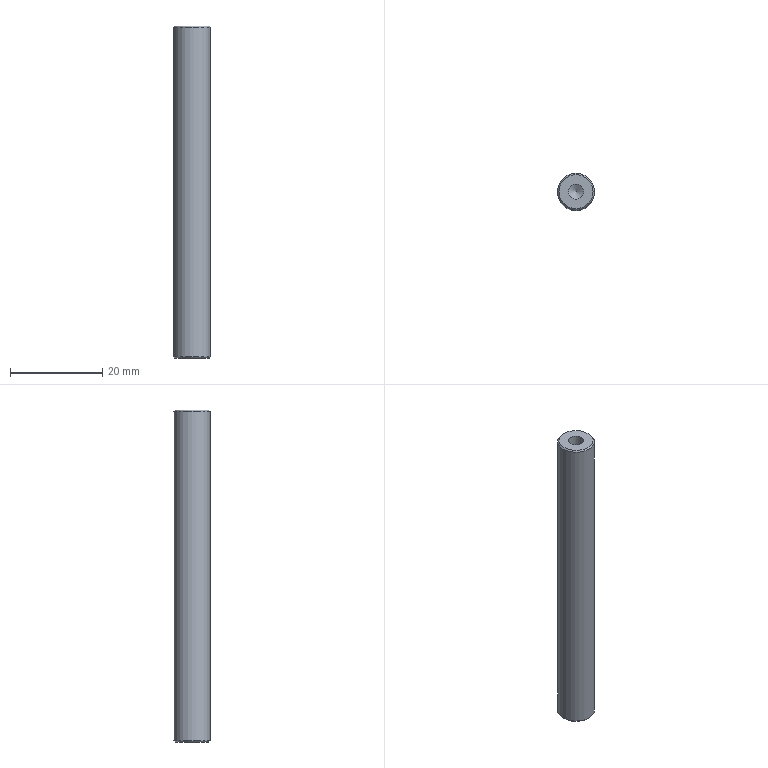Part | NX | 1 solid | 9 faces | box 8 x 8 x 72 mm | volume 3415 mm3 | cone 4 | cylinder 3 | plane 2 | commonest cylinder face diameters 3.3 x2 8 x1
STEP:
#1=CARTESIAN_POINT('',(4.,0.,35.7));
#2=VERTEX_POINT('',#1);
#3=CARTESIAN_POINT('',(0.,0.,35.7));
#4=DIRECTION('',(0.,0.,1.));
#5=DIRECTION('',(1.,0.,0.));
#6=AXIS2_PLACEMENT_3D('',#3,#4,#5);
#7=CIRCLE('',#6,4.);
#8=EDGE_CURVE('',#2,#2,#7,.F.);
#9=ORIENTED_EDGE('',*,*,#8,.T.);
#10=EDGE_LOOP('',(#9));
#11=FACE_BOUND('',#10,.T.);
#12=CARTESIAN_POINT('',(4.,0.,-35.7));
#13=VERTEX_POINT('',#12);
#14=CARTESIAN_POINT('',(0.,0.,-35.7));
#15=DIRECTION('',(0.,0.,1.));
#16=DIRECTION('',(1.,0.,0.));
#17=AXIS2_PLACEMENT_3D('',#14,#15,#16);
#18=CIRCLE('',#17,4.);
#19=EDGE_CURVE('',#13,#13,#18,.T.);
#20=ORIENTED_EDGE('',*,*,#19,.T.);
#21=EDGE_LOOP('',(#20));
#22=FACE_BOUND('',#21,.T.);
#23=CARTESIAN_POINT('',(0.,0.,36.));
#24=DIRECTION('',(0.,0.,-1.));
#25=DIRECTION('',(-1.,0.,0.));
#26=AXIS2_PLACEMENT_3D('',#23,#24,#25);
#27=CYLINDRICAL_SURFACE('',#26,4.);
#28=ADVANCED_FACE('',(#11,#22),#27,.T.);
#29=CARTESIAN_POINT('',(3.7,0.,36.));
#30=VERTEX_POINT('',#29);
#31=CARTESIAN_POINT('',(0.,0.,36.));
#32=DIRECTION('',(0.,0.,1.));
#33=DIRECTION('',(1.,0.,0.));
#34=AXIS2_PLACEMENT_3D('',#31,#32,#33);
#35=CIRCLE('',#34,3.7);
#36=EDGE_CURVE('',#30,#30,#35,.T.);
#37=ORIENTED_EDGE('',*,*,#36,.T.);
#38=EDGE_LOOP('',(#37));
#39=FACE_BOUND('',#38,.T.);
#40=CARTESIAN_POINT('',(1.65,0.,36.));
#41=VERTEX_POINT('',#40);
#42=CARTESIAN_POINT('',(0.,0.,36.));
#43=DIRECTION('',(0.,0.,1.));
#44=DIRECTION('',(1.,0.,0.));
#45=AXIS2_PLACEMENT_3D('',#42,#43,#44);
#46=CIRCLE('',#45,1.65);
#47=EDGE_CURVE('',#41,#41,#46,.T.);
#48=ORIENTED_EDGE('',*,*,#47,.F.);
#49=EDGE_LOOP('',(#48));
#50=FACE_BOUND('',#49,.T.);
#51=CARTESIAN_POINT('',(0.,0.,36.));
#52=DIRECTION('',(0.,0.,1.));
#53=DIRECTION('',(1.,0.,0.));
#54=AXIS2_PLACEMENT_3D('',#51,#52,#53);
#55=PLANE('',#54);
#56=ADVANCED_FACE('',(#39,#50),#55,.T.);
#57=CARTESIAN_POINT('',(3.7,0.,-36.));
#58=VERTEX_POINT('',#57);
#59=CARTESIAN_POINT('',(0.,0.,-36.));
#60=DIRECTION('',(0.,0.,1.));
#61=DIRECTION('',(1.,0.,0.));
#62=AXIS2_PLACEMENT_3D('',#59,#60,#61);
#63=CIRCLE('',#62,3.7);
#64=EDGE_CURVE('',#58,#58,#63,.F.);
#65=ORIENTED_EDGE('',*,*,#64,.T.);
#66=EDGE_LOOP('',(#65));
#67=FACE_BOUND('',#66,.T.);
#68=CARTESIAN_POINT('',(-1.65,0.,-36.));
#69=VERTEX_POINT('',#68);
#70=CARTESIAN_POINT('',(0.,0.,-36.));
#71=DIRECTION('',(0.,0.,-1.));
#72=DIRECTION('',(-1.,0.,0.));
#73=AXIS2_PLACEMENT_3D('',#70,#71,#72);
#74=CIRCLE('',#73,1.65);
#75=EDGE_CURVE('',#69,#69,#74,.T.);
#76=ORIENTED_EDGE('',*,*,#75,.F.);
#77=EDGE_LOOP('',(#76));
#78=FACE_BOUND('',#77,.T.);
#79=CARTESIAN_POINT('',(0.,0.,-36.));
#80=DIRECTION('',(0.,0.,1.));
#81=DIRECTION('',(1.,0.,0.));
#82=AXIS2_PLACEMENT_3D('',#79,#80,#81);
#83=PLANE('',#82);
#84=ADVANCED_FACE('',(#67,#78),#83,.F.);
#85=CARTESIAN_POINT('',(0.,0.,-23.509));
#86=VERTEX_POINT('',#85);
#87=VERTEX_LOOP('',#86);
#88=FACE_BOUND('',#87,.T.);
#89=CARTESIAN_POINT('',(-1.65,0.,-24.5));
#90=VERTEX_POINT('',#89);
#91=CARTESIAN_POINT('',(0.,0.,-24.5));
#92=DIRECTION('',(0.,0.,-1.));
#93=DIRECTION('',(-1.,0.,0.));
#94=AXIS2_PLACEMENT_3D('',#91,#92,#93);
#95=CIRCLE('',#94,1.65);
#96=EDGE_CURVE('',#90,#90,#95,.T.);
#97=ORIENTED_EDGE('',*,*,#96,.T.);
#98=EDGE_LOOP('',(#97));
#99=FACE_BOUND('',#98,.T.);
#100=CARTESIAN_POINT('',(0.,0.,-24.5));
#101=DIRECTION('',(0.,0.,-1.));
#102=DIRECTION('',(-1.,0.,0.));
#103=AXIS2_PLACEMENT_3D('',#100,#101,#102);
#104=CONICAL_SURFACE('',#103,1.65,1.03);
#105=ADVANCED_FACE('',(#88,#99),#104,.F.);
#106=ORIENTED_EDGE('',*,*,#96,.F.);
#107=EDGE_LOOP('',(#106));
#108=FACE_BOUND('',#107,.T.);
#109=ORIENTED_EDGE('',*,*,#75,.T.);
#110=EDGE_LOOP('',(#109));
#111=FACE_BOUND('',#110,.T.);
#112=CARTESIAN_POINT('',(0.,0.,-36.));
#113=DIRECTION('',(0.,0.,-1.));
#114=DIRECTION('',(-1.,0.,0.));
#115=AXIS2_PLACEMENT_3D('',#112,#113,#114);
#116=CYLINDRICAL_SURFACE('',#115,1.65);
#117=ADVANCED_FACE('',(#108,#111),#116,.F.);
#118=CARTESIAN_POINT('',(0.,0.,23.509));
#119=VERTEX_POINT('',#118);
#120=VERTEX_LOOP('',#119);
#121=FACE_BOUND('',#120,.T.);
#122=CARTESIAN_POINT('',(1.65,0.,24.5));
#123=VERTEX_POINT('',#122);
#124=CARTESIAN_POINT('',(0.,0.,24.5));
#125=DIRECTION('',(0.,0.,1.));
#126=DIRECTION('',(1.,0.,0.));
#127=AXIS2_PLACEMENT_3D('',#124,#125,#126);
#128=CIRCLE('',#127,1.65);
#129=EDGE_CURVE('',#123,#123,#128,.T.);
#130=ORIENTED_EDGE('',*,*,#129,.T.);
#131=EDGE_LOOP('',(#130));
#132=FACE_BOUND('',#131,.T.);
#133=CARTESIAN_POINT('',(0.,0.,24.5));
#134=DIRECTION('',(0.,0.,1.));
#135=DIRECTION('',(1.,0.,0.));
#136=AXIS2_PLACEMENT_3D('',#133,#134,#135);
#137=CONICAL_SURFACE('',#136,1.65,1.03);
#138=ADVANCED_FACE('',(#121,#132),#137,.F.);
#139=ORIENTED_EDGE('',*,*,#129,.F.);
#140=EDGE_LOOP('',(#139));
#141=FACE_BOUND('',#140,.T.);
#142=ORIENTED_EDGE('',*,*,#47,.T.);
#143=EDGE_LOOP('',(#142));
#144=FACE_BOUND('',#143,.T.);
#145=CARTESIAN_POINT('',(0.,0.,36.));
#146=DIRECTION('',(0.,0.,1.));
#147=DIRECTION('',(1.,0.,0.));
#148=AXIS2_PLACEMENT_3D('',#145,#146,#147);
#149=CYLINDRICAL_SURFACE('',#148,1.65);
#150=ADVANCED_FACE('',(#141,#144),#149,.F.);
#151=ORIENTED_EDGE('',*,*,#8,.F.);
#152=EDGE_LOOP('',(#151));
#153=FACE_BOUND('',#152,.T.);
#154=ORIENTED_EDGE('',*,*,#36,.F.);
#155=EDGE_LOOP('',(#154));
#156=FACE_BOUND('',#155,.T.);
#157=CARTESIAN_POINT('',(0.,0.,36.));
#158=DIRECTION('',(0.,0.,-1.));
#159=DIRECTION('',(-1.,0.,0.));
#160=AXIS2_PLACEMENT_3D('',#157,#158,#159);
#161=CONICAL_SURFACE('',#160,3.7,0.7854);
#162=ADVANCED_FACE('',(#153,#156),#161,.T.);
#163=ORIENTED_EDGE('',*,*,#64,.F.);
#164=EDGE_LOOP('',(#163));
#165=FACE_BOUND('',#164,.T.);
#166=ORIENTED_EDGE('',*,*,#19,.F.);
#167=EDGE_LOOP('',(#166));
#168=FACE_BOUND('',#167,.T.);
#169=CARTESIAN_POINT('',(0.,0.,-35.7));
#170=DIRECTION('',(0.,0.,1.));
#171=DIRECTION('',(1.,0.,0.));
#172=AXIS2_PLACEMENT_3D('',#169,#170,#171);
#173=CONICAL_SURFACE('',#172,4.,0.7854);
#174=ADVANCED_FACE('',(#165,#168),#173,.T.);
#175=CLOSED_SHELL('',(#28,#56,#84,#105,#117,#138,#150,#162,#174));
#176=MANIFOLD_SOLID_BREP('',#175);
#177=(LENGTH_UNIT()NAMED_UNIT(*)SI_UNIT(.MILLI.,.METRE.));
#178=UNCERTAINTY_MEASURE_WITH_UNIT(LENGTH_MEASURE(0.00001),#177,'','');
#179=(NAMED_UNIT(*)PLANE_ANGLE_UNIT()SI_UNIT($,.RADIAN.));
#180=(NAMED_UNIT(*)SI_UNIT($,.STERADIAN.)SOLID_ANGLE_UNIT());
#181=(GEOMETRIC_REPRESENTATION_CONTEXT(3)GLOBAL_UNCERTAINTY_ASSIGNED_CONTEXT((#178))GLOBAL_UNIT_ASSIGNED_CONTEXT((#177,#179,#180))REPRESENTATION_CONTEXT('',''));
#182=ADVANCED_BREP_SHAPE_REPRESENTATION('',(#176),#181);